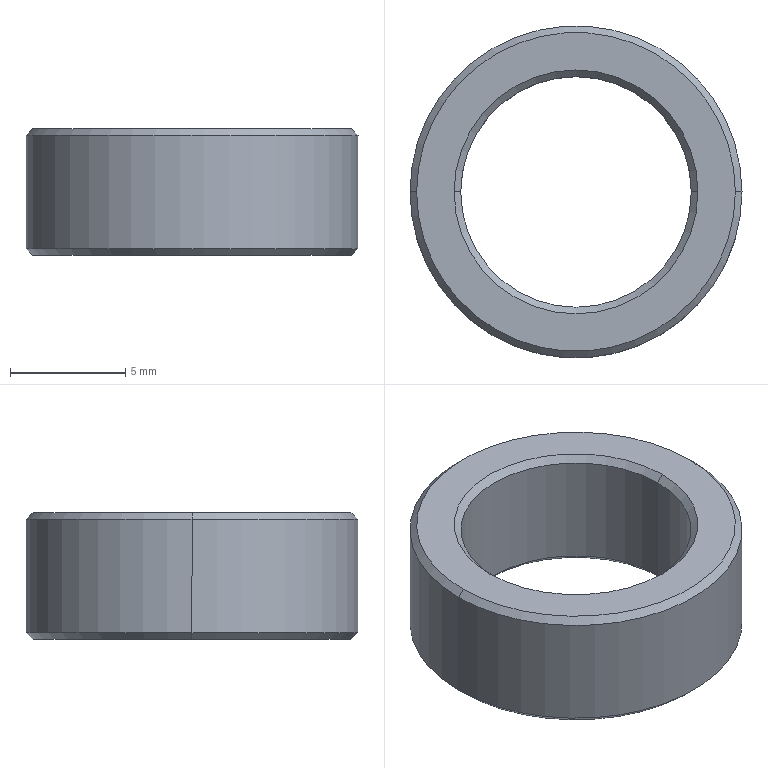Part | SolidWorks | features BaseBody 1 | 1 solid | 14 faces | box 14.4 x 14.4 x 5.5 mm | volume 457.404 mm3 | cone 8 | cylinder 4 | plane 2 | commonest cylinder face diameters 10 x2 14.4 x2
STEP:
#1=CARTESIAN_POINT('',(7.2,0.,-2.462));
#2=VERTEX_POINT('',#1);
#3=CARTESIAN_POINT('',(-7.2,0.,-2.462));
#4=VERTEX_POINT('',#3);
#5=CARTESIAN_POINT('',(0.,0.,-2.462));
#6=DIRECTION('',(0.,0.,1.));
#7=DIRECTION('',(1.,0.,0.));
#8=AXIS2_PLACEMENT_3D('',#5,#6,#7);
#9=CIRCLE('',#8,7.2);
#10=EDGE_CURVE('',#2,#4,#9,.T.);
#11=ORIENTED_EDGE('',*,*,#10,.T.);
#12=CARTESIAN_POINT('',(-7.2,0.,2.462));
#13=VERTEX_POINT('',#12);
#14=CARTESIAN_POINT('',(-7.2,0.,-50.));
#15=DIRECTION('',(0.,0.,1.));
#16=VECTOR('',#15,1000.);
#17=LINE('',#14,#16);
#18=EDGE_CURVE('',#4,#13,#17,.T.);
#19=ORIENTED_EDGE('',*,*,#18,.T.);
#20=CARTESIAN_POINT('',(7.2,0.,2.462));
#21=VERTEX_POINT('',#20);
#22=CARTESIAN_POINT('',(0.,0.,2.462));
#23=DIRECTION('',(0.,0.,-1.));
#24=DIRECTION('',(1.,0.,0.));
#25=AXIS2_PLACEMENT_3D('',#22,#23,#24);
#26=CIRCLE('',#25,7.2);
#27=EDGE_CURVE('',#13,#21,#26,.T.);
#28=ORIENTED_EDGE('',*,*,#27,.T.);
#29=CARTESIAN_POINT('',(7.2,0.,-50.));
#30=DIRECTION('',(0.,0.,1.));
#31=VECTOR('',#30,1000.);
#32=LINE('',#29,#31);
#33=EDGE_CURVE('',#2,#21,#32,.T.);
#34=ORIENTED_EDGE('',*,*,#33,.F.);
#35=EDGE_LOOP('',(#11,#19,#28,#34));
#36=FACE_OUTER_BOUND('',#35,.T.);
#37=CARTESIAN_POINT('',(0.,0.,-50.));
#38=DIRECTION('',(0.,0.,1.));
#39=DIRECTION('',(1.,0.,0.));
#40=AXIS2_PLACEMENT_3D('',#37,#38,#39);
#41=CYLINDRICAL_SURFACE('',#40,7.2);
#42=ADVANCED_FACE('',(#36),#41,.T.);
#43=CARTESIAN_POINT('',(6.912,0.,-2.75));
#44=VERTEX_POINT('',#43);
#45=CARTESIAN_POINT('',(-6.912,0.,-2.75));
#46=VERTEX_POINT('',#45);
#47=CARTESIAN_POINT('',(0.,0.,-2.75));
#48=DIRECTION('',(0.,0.,1.));
#49=DIRECTION('',(1.,0.,0.));
#50=AXIS2_PLACEMENT_3D('',#47,#48,#49);
#51=CIRCLE('',#50,6.912);
#52=EDGE_CURVE('',#44,#46,#51,.T.);
#53=ORIENTED_EDGE('',*,*,#52,.T.);
#54=CARTESIAN_POINT('',(-7.2,0.,-2.462));
#55=DIRECTION('',(-0.7071,0.,0.7071));
#56=VECTOR('',#55,1000.);
#57=LINE('',#54,#56);
#58=EDGE_CURVE('',#46,#4,#57,.T.);
#59=ORIENTED_EDGE('',*,*,#58,.T.);
#60=ORIENTED_EDGE('',*,*,#10,.F.);
#61=CARTESIAN_POINT('',(7.2,0.,-2.462));
#62=DIRECTION('',(0.7071,0.,0.7071));
#63=VECTOR('',#62,1000.);
#64=LINE('',#61,#63);
#65=EDGE_CURVE('',#44,#2,#64,.T.);
#66=ORIENTED_EDGE('',*,*,#65,.F.);
#67=EDGE_LOOP('',(#53,#59,#60,#66));
#68=FACE_OUTER_BOUND('',#67,.T.);
#69=CARTESIAN_POINT('',(0.,0.,-2.462));
#70=DIRECTION('',(0.,0.,1.));
#71=DIRECTION('',(1.,0.,0.));
#72=AXIS2_PLACEMENT_3D('',#69,#70,#71);
#73=CONICAL_SURFACE('',#72,7.2,0.7854);
#74=ADVANCED_FACE('',(#68),#73,.T.);
#75=CARTESIAN_POINT('',(-6.912,0.,2.75));
#76=VERTEX_POINT('',#75);
#77=CARTESIAN_POINT('',(6.912,0.,2.75));
#78=VERTEX_POINT('',#77);
#79=CARTESIAN_POINT('',(0.,0.,2.75));
#80=DIRECTION('',(0.,0.,-1.));
#81=DIRECTION('',(-1.,0.,0.));
#82=AXIS2_PLACEMENT_3D('',#79,#80,#81);
#83=CIRCLE('',#82,6.912);
#84=EDGE_CURVE('',#76,#78,#83,.T.);
#85=ORIENTED_EDGE('',*,*,#84,.T.);
#86=CARTESIAN_POINT('',(7.2,0.,2.462));
#87=DIRECTION('',(0.7071,0.,-0.7071));
#88=VECTOR('',#87,1000.);
#89=LINE('',#86,#88);
#90=EDGE_CURVE('',#78,#21,#89,.T.);
#91=ORIENTED_EDGE('',*,*,#90,.T.);
#92=ORIENTED_EDGE('',*,*,#27,.F.);
#93=CARTESIAN_POINT('',(-7.2,0.,2.462));
#94=DIRECTION('',(-0.7071,0.,-0.7071));
#95=VECTOR('',#94,1000.);
#96=LINE('',#93,#95);
#97=EDGE_CURVE('',#76,#13,#96,.T.);
#98=ORIENTED_EDGE('',*,*,#97,.F.);
#99=EDGE_LOOP('',(#85,#91,#92,#98));
#100=FACE_OUTER_BOUND('',#99,.T.);
#101=CARTESIAN_POINT('',(0.,0.,2.462));
#102=DIRECTION('',(0.,0.,-1.));
#103=DIRECTION('',(-1.,0.,0.));
#104=AXIS2_PLACEMENT_3D('',#101,#102,#103);
#105=CONICAL_SURFACE('',#104,7.2,0.7854);
#106=ADVANCED_FACE('',(#100),#105,.T.);
#107=CARTESIAN_POINT('',(5.,0.,-2.462));
#108=VERTEX_POINT('',#107);
#109=CARTESIAN_POINT('',(-5.,0.,-2.462));
#110=VERTEX_POINT('',#109);
#111=CARTESIAN_POINT('',(0.,0.,-2.462));
#112=DIRECTION('',(0.,0.,-1.));
#113=DIRECTION('',(-1.,0.,0.));
#114=AXIS2_PLACEMENT_3D('',#111,#112,#113);
#115=CIRCLE('',#114,5.);
#116=EDGE_CURVE('',#108,#110,#115,.T.);
#117=ORIENTED_EDGE('',*,*,#116,.F.);
#118=CARTESIAN_POINT('',(5.288,0.,-2.75));
#119=VERTEX_POINT('',#118);
#120=CARTESIAN_POINT('',(5.288,0.,-2.75));
#121=DIRECTION('',(0.7071,0.,-0.7071));
#122=VECTOR('',#121,1000.);
#123=LINE('',#120,#122);
#124=EDGE_CURVE('',#108,#119,#123,.T.);
#125=ORIENTED_EDGE('',*,*,#124,.T.);
#126=CARTESIAN_POINT('',(-5.288,0.,-2.75));
#127=VERTEX_POINT('',#126);
#128=CARTESIAN_POINT('',(0.,0.,-2.75));
#129=DIRECTION('',(0.,0.,1.));
#130=DIRECTION('',(-1.,0.,0.));
#131=AXIS2_PLACEMENT_3D('',#128,#129,#130);
#132=CIRCLE('',#131,5.288);
#133=EDGE_CURVE('',#127,#119,#132,.T.);
#134=ORIENTED_EDGE('',*,*,#133,.F.);
#135=CARTESIAN_POINT('',(-5.288,0.,-2.75));
#136=DIRECTION('',(-0.7071,0.,-0.7071));
#137=VECTOR('',#136,1000.);
#138=LINE('',#135,#137);
#139=EDGE_CURVE('',#110,#127,#138,.T.);
#140=ORIENTED_EDGE('',*,*,#139,.F.);
#141=EDGE_LOOP('',(#117,#125,#134,#140));
#142=FACE_OUTER_BOUND('',#141,.T.);
#143=CARTESIAN_POINT('',(0.,0.,-2.75));
#144=DIRECTION('',(0.,0.,-1.));
#145=DIRECTION('',(-1.,0.,0.));
#146=AXIS2_PLACEMENT_3D('',#143,#144,#145);
#147=CONICAL_SURFACE('',#146,5.288,0.7854);
#148=ADVANCED_FACE('',(#142),#147,.F.);
#149=CARTESIAN_POINT('',(-5.,0.,2.462));
#150=VERTEX_POINT('',#149);
#151=CARTESIAN_POINT('',(5.,0.,2.462));
#152=VERTEX_POINT('',#151);
#153=CARTESIAN_POINT('',(0.,0.,2.462));
#154=DIRECTION('',(0.,0.,1.));
#155=DIRECTION('',(1.,0.,0.));
#156=AXIS2_PLACEMENT_3D('',#153,#154,#155);
#157=CIRCLE('',#156,5.);
#158=EDGE_CURVE('',#150,#152,#157,.T.);
#159=ORIENTED_EDGE('',*,*,#158,.F.);
#160=CARTESIAN_POINT('',(-5.288,0.,2.75));
#161=VERTEX_POINT('',#160);
#162=CARTESIAN_POINT('',(-5.288,0.,2.75));
#163=DIRECTION('',(-0.7071,0.,0.7071));
#164=VECTOR('',#163,1000.);
#165=LINE('',#162,#164);
#166=EDGE_CURVE('',#150,#161,#165,.T.);
#167=ORIENTED_EDGE('',*,*,#166,.T.);
#168=CARTESIAN_POINT('',(5.288,0.,2.75));
#169=VERTEX_POINT('',#168);
#170=CARTESIAN_POINT('',(0.,0.,2.75));
#171=DIRECTION('',(0.,0.,-1.));
#172=DIRECTION('',(1.,0.,0.));
#173=AXIS2_PLACEMENT_3D('',#170,#171,#172);
#174=CIRCLE('',#173,5.288);
#175=EDGE_CURVE('',#169,#161,#174,.T.);
#176=ORIENTED_EDGE('',*,*,#175,.F.);
#177=CARTESIAN_POINT('',(5.288,0.,2.75));
#178=DIRECTION('',(0.7071,0.,0.7071));
#179=VECTOR('',#178,1000.);
#180=LINE('',#177,#179);
#181=EDGE_CURVE('',#152,#169,#180,.T.);
#182=ORIENTED_EDGE('',*,*,#181,.F.);
#183=EDGE_LOOP('',(#159,#167,#176,#182));
#184=FACE_OUTER_BOUND('',#183,.T.);
#185=CARTESIAN_POINT('',(0.,0.,2.75));
#186=DIRECTION('',(0.,0.,1.));
#187=DIRECTION('',(1.,0.,0.));
#188=AXIS2_PLACEMENT_3D('',#185,#186,#187);
#189=CONICAL_SURFACE('',#188,5.288,0.7854);
#190=ADVANCED_FACE('',(#184),#189,.F.);
#191=ORIENTED_EDGE('',*,*,#116,.T.);
#192=CARTESIAN_POINT('',(-5.,0.,-50.));
#193=DIRECTION('',(0.,0.,1.));
#194=VECTOR('',#193,1000.);
#195=LINE('',#192,#194);
#196=EDGE_CURVE('',#110,#150,#195,.T.);
#197=ORIENTED_EDGE('',*,*,#196,.T.);
#198=ORIENTED_EDGE('',*,*,#158,.T.);
#199=CARTESIAN_POINT('',(5.,0.,-50.));
#200=DIRECTION('',(0.,0.,1.));
#201=VECTOR('',#200,1000.);
#202=LINE('',#199,#201);
#203=EDGE_CURVE('',#108,#152,#202,.T.);
#204=ORIENTED_EDGE('',*,*,#203,.F.);
#205=EDGE_LOOP('',(#191,#197,#198,#204));
#206=FACE_OUTER_BOUND('',#205,.T.);
#207=CARTESIAN_POINT('',(0.,0.,-50.));
#208=DIRECTION('',(0.,0.,1.));
#209=DIRECTION('',(1.,0.,0.));
#210=AXIS2_PLACEMENT_3D('',#207,#208,#209);
#211=CYLINDRICAL_SURFACE('',#210,5.);
#212=ADVANCED_FACE('',(#206),#211,.F.);
#213=ORIENTED_EDGE('',*,*,#18,.F.);
#214=CARTESIAN_POINT('',(0.,0.,-2.462));
#215=DIRECTION('',(0.,0.,1.));
#216=DIRECTION('',(1.,0.,0.));
#217=AXIS2_PLACEMENT_3D('',#214,#215,#216);
#218=CIRCLE('',#217,7.2);
#219=EDGE_CURVE('',#4,#2,#218,.T.);
#220=ORIENTED_EDGE('',*,*,#219,.T.);
#221=ORIENTED_EDGE('',*,*,#33,.T.);
#222=CARTESIAN_POINT('',(0.,0.,2.462));
#223=DIRECTION('',(0.,0.,-1.));
#224=DIRECTION('',(1.,0.,0.));
#225=AXIS2_PLACEMENT_3D('',#222,#223,#224);
#226=CIRCLE('',#225,7.2);
#227=EDGE_CURVE('',#21,#13,#226,.T.);
#228=ORIENTED_EDGE('',*,*,#227,.T.);
#229=EDGE_LOOP('',(#213,#220,#221,#228));
#230=FACE_OUTER_BOUND('',#229,.T.);
#231=CARTESIAN_POINT('',(0.,0.,-50.));
#232=DIRECTION('',(0.,0.,1.));
#233=DIRECTION('',(1.,0.,0.));
#234=AXIS2_PLACEMENT_3D('',#231,#232,#233);
#235=CYLINDRICAL_SURFACE('',#234,7.2);
#236=ADVANCED_FACE('',(#230),#235,.T.);
#237=ORIENTED_EDGE('',*,*,#58,.F.);
#238=CARTESIAN_POINT('',(0.,0.,-2.75));
#239=DIRECTION('',(0.,0.,1.));
#240=DIRECTION('',(1.,0.,0.));
#241=AXIS2_PLACEMENT_3D('',#238,#239,#240);
#242=CIRCLE('',#241,6.912);
#243=EDGE_CURVE('',#46,#44,#242,.T.);
#244=ORIENTED_EDGE('',*,*,#243,.T.);
#245=ORIENTED_EDGE('',*,*,#65,.T.);
#246=ORIENTED_EDGE('',*,*,#219,.F.);
#247=EDGE_LOOP('',(#237,#244,#245,#246));
#248=FACE_OUTER_BOUND('',#247,.T.);
#249=CARTESIAN_POINT('',(0.,0.,-2.462));
#250=DIRECTION('',(0.,0.,1.));
#251=DIRECTION('',(1.,0.,0.));
#252=AXIS2_PLACEMENT_3D('',#249,#250,#251);
#253=CONICAL_SURFACE('',#252,7.2,0.7854);
#254=ADVANCED_FACE('',(#248),#253,.T.);
#255=ORIENTED_EDGE('',*,*,#90,.F.);
#256=CARTESIAN_POINT('',(0.,0.,2.75));
#257=DIRECTION('',(0.,0.,-1.));
#258=DIRECTION('',(-1.,0.,0.));
#259=AXIS2_PLACEMENT_3D('',#256,#257,#258);
#260=CIRCLE('',#259,6.912);
#261=EDGE_CURVE('',#78,#76,#260,.T.);
#262=ORIENTED_EDGE('',*,*,#261,.T.);
#263=ORIENTED_EDGE('',*,*,#97,.T.);
#264=ORIENTED_EDGE('',*,*,#227,.F.);
#265=EDGE_LOOP('',(#255,#262,#263,#264));
#266=FACE_OUTER_BOUND('',#265,.T.);
#267=CARTESIAN_POINT('',(0.,0.,2.462));
#268=DIRECTION('',(0.,0.,-1.));
#269=DIRECTION('',(-1.,0.,0.));
#270=AXIS2_PLACEMENT_3D('',#267,#268,#269);
#271=CONICAL_SURFACE('',#270,7.2,0.7854);
#272=ADVANCED_FACE('',(#266),#271,.T.);
#273=ORIENTED_EDGE('',*,*,#133,.T.);
#274=CARTESIAN_POINT('',(0.,0.,-2.75));
#275=DIRECTION('',(0.,0.,1.));
#276=DIRECTION('',(-1.,0.,0.));
#277=AXIS2_PLACEMENT_3D('',#274,#275,#276);
#278=CIRCLE('',#277,5.288);
#279=EDGE_CURVE('',#119,#127,#278,.T.);
#280=ORIENTED_EDGE('',*,*,#279,.T.);
#281=EDGE_LOOP('',(#273,#280));
#282=FACE_BOUND('',#281,.T.);
#283=ORIENTED_EDGE('',*,*,#52,.F.);
#284=ORIENTED_EDGE('',*,*,#243,.F.);
#285=EDGE_LOOP('',(#283,#284));
#286=FACE_OUTER_BOUND('',#285,.T.);
#287=CARTESIAN_POINT('',(0.,5.288,-2.75));
#288=DIRECTION('',(0.,0.,-1.));
#289=DIRECTION('',(-1.,0.,0.));
#290=AXIS2_PLACEMENT_3D('',#287,#288,#289);
#291=PLANE('',#290);
#292=ADVANCED_FACE('',(#282,#286),#291,.T.);
#293=ORIENTED_EDGE('',*,*,#84,.F.);
#294=ORIENTED_EDGE('',*,*,#261,.F.);
#295=EDGE_LOOP('',(#293,#294));
#296=FACE_OUTER_BOUND('',#295,.T.);
#297=ORIENTED_EDGE('',*,*,#175,.T.);
#298=CARTESIAN_POINT('',(0.,0.,2.75));
#299=DIRECTION('',(0.,0.,-1.));
#300=DIRECTION('',(1.,0.,0.));
#301=AXIS2_PLACEMENT_3D('',#298,#299,#300);
#302=CIRCLE('',#301,5.288);
#303=EDGE_CURVE('',#161,#169,#302,.T.);
#304=ORIENTED_EDGE('',*,*,#303,.T.);
#305=EDGE_LOOP('',(#297,#304));
#306=FACE_BOUND('',#305,.T.);
#307=CARTESIAN_POINT('',(0.,6.912,2.75));
#308=DIRECTION('',(0.,0.,1.));
#309=DIRECTION('',(1.,0.,0.));
#310=AXIS2_PLACEMENT_3D('',#307,#308,#309);
#311=PLANE('',#310);
#312=ADVANCED_FACE('',(#296,#306),#311,.T.);
#313=ORIENTED_EDGE('',*,*,#124,.F.);
#314=CARTESIAN_POINT('',(0.,0.,-2.462));
#315=DIRECTION('',(0.,0.,-1.));
#316=DIRECTION('',(-1.,0.,0.));
#317=AXIS2_PLACEMENT_3D('',#314,#315,#316);
#318=CIRCLE('',#317,5.);
#319=EDGE_CURVE('',#110,#108,#318,.T.);
#320=ORIENTED_EDGE('',*,*,#319,.F.);
#321=ORIENTED_EDGE('',*,*,#139,.T.);
#322=ORIENTED_EDGE('',*,*,#279,.F.);
#323=EDGE_LOOP('',(#313,#320,#321,#322));
#324=FACE_OUTER_BOUND('',#323,.T.);
#325=CARTESIAN_POINT('',(0.,0.,-2.75));
#326=DIRECTION('',(0.,0.,-1.));
#327=DIRECTION('',(-1.,0.,0.));
#328=AXIS2_PLACEMENT_3D('',#325,#326,#327);
#329=CONICAL_SURFACE('',#328,5.288,0.7854);
#330=ADVANCED_FACE('',(#324),#329,.F.);
#331=ORIENTED_EDGE('',*,*,#166,.F.);
#332=CARTESIAN_POINT('',(0.,0.,2.462));
#333=DIRECTION('',(0.,0.,1.));
#334=DIRECTION('',(1.,0.,0.));
#335=AXIS2_PLACEMENT_3D('',#332,#333,#334);
#336=CIRCLE('',#335,5.);
#337=EDGE_CURVE('',#152,#150,#336,.T.);
#338=ORIENTED_EDGE('',*,*,#337,.F.);
#339=ORIENTED_EDGE('',*,*,#181,.T.);
#340=ORIENTED_EDGE('',*,*,#303,.F.);
#341=EDGE_LOOP('',(#331,#338,#339,#340));
#342=FACE_OUTER_BOUND('',#341,.T.);
#343=CARTESIAN_POINT('',(0.,0.,2.75));
#344=DIRECTION('',(0.,0.,1.));
#345=DIRECTION('',(1.,0.,0.));
#346=AXIS2_PLACEMENT_3D('',#343,#344,#345);
#347=CONICAL_SURFACE('',#346,5.288,0.7854);
#348=ADVANCED_FACE('',(#342),#347,.F.);
#349=ORIENTED_EDGE('',*,*,#196,.F.);
#350=ORIENTED_EDGE('',*,*,#319,.T.);
#351=ORIENTED_EDGE('',*,*,#203,.T.);
#352=ORIENTED_EDGE('',*,*,#337,.T.);
#353=EDGE_LOOP('',(#349,#350,#351,#352));
#354=FACE_OUTER_BOUND('',#353,.T.);
#355=CARTESIAN_POINT('',(0.,0.,-50.));
#356=DIRECTION('',(0.,0.,1.));
#357=DIRECTION('',(1.,0.,0.));
#358=AXIS2_PLACEMENT_3D('',#355,#356,#357);
#359=CYLINDRICAL_SURFACE('',#358,5.);
#360=ADVANCED_FACE('',(#354),#359,.F.);
#361=CLOSED_SHELL('',(#42,#74,#106,#148,#190,#212,#236,#254,#272,#292,#312,#330,#348,#360));
#362=MANIFOLD_SOLID_BREP('',#361);
#363=CARTESIAN_POINT('',(0.,0.,0.));
#364=DIRECTION('',(0.,0.,1.));
#365=DIRECTION('',(1.,0.,0.));
#366=AXIS2_PLACEMENT_3D('',#363,#364,#365);
#367=(LENGTH_UNIT()NAMED_UNIT(*)SI_UNIT(.MILLI.,.METRE.));
#368=UNCERTAINTY_MEASURE_WITH_UNIT(LENGTH_MEASURE(0.00001),#367,'','');
#369=(NAMED_UNIT(*)PLANE_ANGLE_UNIT()SI_UNIT($,.RADIAN.));
#370=(NAMED_UNIT(*)SI_UNIT($,.STERADIAN.)SOLID_ANGLE_UNIT());
#371=(GEOMETRIC_REPRESENTATION_CONTEXT(3)GLOBAL_UNCERTAINTY_ASSIGNED_CONTEXT((#368))GLOBAL_UNIT_ASSIGNED_CONTEXT((#367,#369,#370))REPRESENTATION_CONTEXT('',''));
#372=ADVANCED_BREP_SHAPE_REPRESENTATION('',(#362,#366),#371);